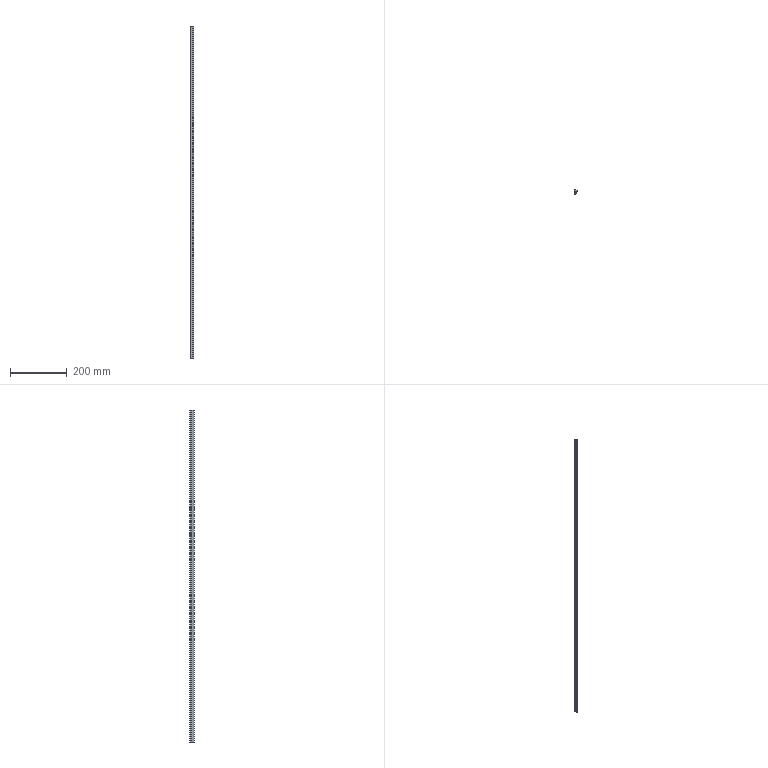Part | SolidWorks | features BaseBody 1, MoveFace 1 | 1 solid | 20 faces | box 10.8 x 17.5 x 1171 mm | volume 92275 mm3 | cylinder 11 | plane 9 | commonest cylinder face diameters 1.6 x2 14 x2 0.4 x1 0.6 x1 0.8 x1 2.6 x1
STEP:
#1=CARTESIAN_POINT('',(-3.236,-11.055,1071.));
#2=VERTEX_POINT('',#1);
#3=CARTESIAN_POINT('',(-4.3,-10.3,1071.));
#4=VERTEX_POINT('',#3);
#5=CARTESIAN_POINT('',(-3.5,-10.3,1071.));
#6=DIRECTION('',(0.,0.,-1.));
#7=DIRECTION('',(1.,0.,0.));
#8=AXIS2_PLACEMENT_3D('',#5,#6,#7);
#9=CIRCLE('',#8,0.8);
#10=EDGE_CURVE('',#2,#4,#9,.T.);
#11=ORIENTED_EDGE('',*,*,#10,.T.);
#12=CARTESIAN_POINT('',(-4.3,-10.3,-100.));
#13=VERTEX_POINT('',#12);
#14=CARTESIAN_POINT('',(-4.3,-10.3,-100.));
#15=DIRECTION('',(0.,0.,-1.));
#16=VECTOR('',#15,1000.);
#17=LINE('',#14,#16);
#18=EDGE_CURVE('',#4,#13,#17,.T.);
#19=ORIENTED_EDGE('',*,*,#18,.T.);
#20=CARTESIAN_POINT('',(-3.236,-11.055,-100.));
#21=VERTEX_POINT('',#20);
#22=CARTESIAN_POINT('',(-3.5,-10.3,-100.));
#23=DIRECTION('',(0.,0.,1.));
#24=DIRECTION('',(-1.,0.,0.));
#25=AXIS2_PLACEMENT_3D('',#22,#23,#24);
#26=CIRCLE('',#25,0.8);
#27=EDGE_CURVE('',#13,#21,#26,.T.);
#28=ORIENTED_EDGE('',*,*,#27,.T.);
#29=CARTESIAN_POINT('',(-3.236,-11.055,-100.));
#30=DIRECTION('',(0.,0.,-1.));
#31=VECTOR('',#30,1000.);
#32=LINE('',#29,#31);
#33=EDGE_CURVE('',#2,#21,#32,.T.);
#34=ORIENTED_EDGE('',*,*,#33,.F.);
#35=EDGE_LOOP('',(#11,#19,#28,#34));
#36=FACE_OUTER_BOUND('',#35,.T.);
#37=CARTESIAN_POINT('',(-3.5,-10.3,-100.));
#38=DIRECTION('',(0.,0.,-1.));
#39=DIRECTION('',(-1.,0.,0.));
#40=AXIS2_PLACEMENT_3D('',#37,#38,#39);
#41=CYLINDRICAL_SURFACE('',#40,0.8);
#42=ADVANCED_FACE('',(#36),#41,.T.);
#43=CARTESIAN_POINT('',(1.184,-6.397,-100.));
#44=VERTEX_POINT('',#43);
#45=CARTESIAN_POINT('',(-5.702,-4.29,-100.));
#46=DIRECTION('',(0.,0.,1.));
#47=DIRECTION('',(-1.,0.,0.));
#48=AXIS2_PLACEMENT_3D('',#45,#46,#47);
#49=CIRCLE('',#48,7.201);
#50=EDGE_CURVE('',#21,#44,#49,.T.);
#51=ORIENTED_EDGE('',*,*,#50,.T.);
#52=CARTESIAN_POINT('',(1.184,-6.397,1071.));
#53=VERTEX_POINT('',#52);
#54=CARTESIAN_POINT('',(1.184,-6.397,-100.));
#55=DIRECTION('',(0.,0.,1.));
#56=VECTOR('',#55,1000.);
#57=LINE('',#54,#56);
#58=EDGE_CURVE('',#44,#53,#57,.T.);
#59=ORIENTED_EDGE('',*,*,#58,.T.);
#60=CARTESIAN_POINT('',(-5.702,-4.29,1071.));
#61=DIRECTION('',(0.,0.,-1.));
#62=DIRECTION('',(1.,0.,0.));
#63=AXIS2_PLACEMENT_3D('',#60,#61,#62);
#64=CIRCLE('',#63,7.201);
#65=EDGE_CURVE('',#53,#2,#64,.T.);
#66=ORIENTED_EDGE('',*,*,#65,.T.);
#67=ORIENTED_EDGE('',*,*,#33,.T.);
#68=EDGE_LOOP('',(#51,#59,#66,#67));
#69=FACE_OUTER_BOUND('',#68,.T.);
#70=CARTESIAN_POINT('',(-5.702,-4.29,-100.));
#71=DIRECTION('',(0.,0.,-1.));
#72=DIRECTION('',(-1.,0.,0.));
#73=AXIS2_PLACEMENT_3D('',#70,#71,#72);
#74=CYLINDRICAL_SURFACE('',#73,7.201);
#75=ADVANCED_FACE('',(#69),#74,.T.);
#76=CARTESIAN_POINT('',(0.9,-6.,-100.));
#77=VERTEX_POINT('',#76);
#78=CARTESIAN_POINT('',(0.9,-6.3,-100.));
#79=DIRECTION('',(0.,0.,1.));
#80=DIRECTION('',(-1.,0.,0.));
#81=AXIS2_PLACEMENT_3D('',#78,#79,#80);
#82=CIRCLE('',#81,0.3);
#83=EDGE_CURVE('',#44,#77,#82,.T.);
#84=ORIENTED_EDGE('',*,*,#83,.T.);
#85=CARTESIAN_POINT('',(0.9,-6.,1071.));
#86=VERTEX_POINT('',#85);
#87=CARTESIAN_POINT('',(0.9,-6.,-100.));
#88=DIRECTION('',(0.,0.,1.));
#89=VECTOR('',#88,1000.);
#90=LINE('',#87,#89);
#91=EDGE_CURVE('',#77,#86,#90,.T.);
#92=ORIENTED_EDGE('',*,*,#91,.T.);
#93=CARTESIAN_POINT('',(0.9,-6.3,1071.));
#94=DIRECTION('',(0.,0.,-1.));
#95=DIRECTION('',(1.,0.,0.));
#96=AXIS2_PLACEMENT_3D('',#93,#94,#95);
#97=CIRCLE('',#96,0.3);
#98=EDGE_CURVE('',#86,#53,#97,.T.);
#99=ORIENTED_EDGE('',*,*,#98,.T.);
#100=ORIENTED_EDGE('',*,*,#58,.F.);
#101=EDGE_LOOP('',(#84,#92,#99,#100));
#102=FACE_OUTER_BOUND('',#101,.T.);
#103=CARTESIAN_POINT('',(0.9,-6.3,-100.));
#104=DIRECTION('',(0.,0.,-1.));
#105=DIRECTION('',(-1.,0.,0.));
#106=AXIS2_PLACEMENT_3D('',#103,#104,#105);
#107=CYLINDRICAL_SURFACE('',#106,0.3);
#108=ADVANCED_FACE('',(#102),#107,.T.);
#109=CARTESIAN_POINT('',(-2.5,-0.5,-100.));
#110=VERTEX_POINT('',#109);
#111=CARTESIAN_POINT('',(-2.5,-6.153,-100.));
#112=VERTEX_POINT('',#111);
#113=CARTESIAN_POINT('',(-2.5,-6.397,-100.));
#114=DIRECTION('',(0.,-1.,0.));
#115=VECTOR('',#114,1000.);
#116=LINE('',#113,#115);
#117=EDGE_CURVE('',#110,#112,#116,.T.);
#118=ORIENTED_EDGE('',*,*,#117,.F.);
#119=CARTESIAN_POINT('',(-4.2,1.695,-100.));
#120=VERTEX_POINT('',#119);
#121=CARTESIAN_POINT('',(-1.701,1.875,-100.));
#122=DIRECTION('',(0.,0.,1.));
#123=DIRECTION('',(-1.,0.,0.));
#124=AXIS2_PLACEMENT_3D('',#121,#122,#123);
#125=CIRCLE('',#124,2.506);
#126=EDGE_CURVE('',#120,#110,#125,.T.);
#127=ORIENTED_EDGE('',*,*,#126,.F.);
#128=CARTESIAN_POINT('',(-4.2,5.1,-100.));
#129=VERTEX_POINT('',#128);
#130=CARTESIAN_POINT('',(-4.2,-6.397,-100.));
#131=DIRECTION('',(0.,-1.,0.));
#132=VECTOR('',#131,1000.);
#133=LINE('',#130,#132);
#134=EDGE_CURVE('',#129,#120,#133,.T.);
#135=ORIENTED_EDGE('',*,*,#134,.F.);
#136=CARTESIAN_POINT('',(-2.892,6.4,-100.));
#137=VERTEX_POINT('',#136);
#138=CARTESIAN_POINT('',(-2.9,5.1,-100.));
#139=DIRECTION('',(0.,0.,1.));
#140=DIRECTION('',(-1.,0.,0.));
#141=AXIS2_PLACEMENT_3D('',#138,#139,#140);
#142=CIRCLE('',#141,1.3);
#143=EDGE_CURVE('',#137,#129,#142,.T.);
#144=ORIENTED_EDGE('',*,*,#143,.F.);
#145=CARTESIAN_POINT('',(0.5,5.5,-100.));
#146=VERTEX_POINT('',#145);
#147=CARTESIAN_POINT('',(-2.934,-0.5999,-100.));
#148=DIRECTION('',(0.,0.,1.));
#149=DIRECTION('',(-1.,0.,0.));
#150=AXIS2_PLACEMENT_3D('',#147,#148,#149);
#151=CIRCLE('',#150,7.);
#152=EDGE_CURVE('',#146,#137,#151,.T.);
#153=ORIENTED_EDGE('',*,*,#152,.F.);
#154=CARTESIAN_POINT('',(5.5,1.7,-100.));
#155=VERTEX_POINT('',#154);
#156=CARTESIAN_POINT('',(5.5,1.7,-100.));
#157=DIRECTION('',(-0.7962,0.6051,0.));
#158=VECTOR('',#157,1000.);
#159=LINE('',#156,#158);
#160=EDGE_CURVE('',#155,#146,#159,.T.);
#161=ORIENTED_EDGE('',*,*,#160,.F.);
#162=CARTESIAN_POINT('',(6.458,-0.2215,-100.));
#163=VERTEX_POINT('',#162);
#164=CARTESIAN_POINT('',(6.458,-0.2215,-100.));
#165=DIRECTION('',(-0.4462,0.8949,0.));
#166=VECTOR('',#165,1000.);
#167=LINE('',#164,#166);
#168=EDGE_CURVE('',#163,#155,#167,.T.);
#169=ORIENTED_EDGE('',*,*,#168,.F.);
#170=CARTESIAN_POINT('',(5.895,-0.7433,-100.));
#171=VERTEX_POINT('',#170);
#172=CARTESIAN_POINT('',(6.1,-0.4,-100.));
#173=DIRECTION('',(0.,0.,1.));
#174=DIRECTION('',(-1.,0.,0.));
#175=AXIS2_PLACEMENT_3D('',#172,#173,#174);
#176=CIRCLE('',#175,0.4);
#177=EDGE_CURVE('',#171,#163,#176,.T.);
#178=ORIENTED_EDGE('',*,*,#177,.F.);
#179=CARTESIAN_POINT('',(3.,0.,-100.));
#180=VERTEX_POINT('',#179);
#181=CARTESIAN_POINT('',(2.746,-6.995,-100.));
#182=DIRECTION('',(0.,0.,-1.));
#183=DIRECTION('',(-1.,0.,0.));
#184=AXIS2_PLACEMENT_3D('',#181,#182,#183);
#185=CIRCLE('',#184,7.);
#186=EDGE_CURVE('',#180,#171,#185,.T.);
#187=ORIENTED_EDGE('',*,*,#186,.F.);
#188=CARTESIAN_POINT('',(0.,0.,-100.));
#189=VERTEX_POINT('',#188);
#190=CARTESIAN_POINT('',(-6.814,0.,-100.));
#191=DIRECTION('',(1.,0.,0.));
#192=VECTOR('',#191,1000.);
#193=LINE('',#190,#192);
#194=EDGE_CURVE('',#189,#180,#193,.T.);
#195=ORIENTED_EDGE('',*,*,#194,.F.);
#196=CARTESIAN_POINT('',(0.,-5.8,-100.));
#197=VERTEX_POINT('',#196);
#198=CARTESIAN_POINT('',(0.,-6.397,-100.));
#199=DIRECTION('',(0.,1.,0.));
#200=VECTOR('',#199,1000.);
#201=LINE('',#198,#200);
#202=EDGE_CURVE('',#197,#189,#201,.T.);
#203=ORIENTED_EDGE('',*,*,#202,.F.);
#204=CARTESIAN_POINT('',(0.2,-6.,-100.));
#205=VERTEX_POINT('',#204);
#206=CARTESIAN_POINT('',(0.2,-5.8,-100.));
#207=DIRECTION('',(0.,0.,1.));
#208=DIRECTION('',(-1.,0.,0.));
#209=AXIS2_PLACEMENT_3D('',#206,#207,#208);
#210=CIRCLE('',#209,0.2);
#211=EDGE_CURVE('',#197,#205,#210,.T.);
#212=ORIENTED_EDGE('',*,*,#211,.T.);
#213=CARTESIAN_POINT('',(-6.814,-6.,-100.));
#214=DIRECTION('',(-1.,0.,0.));
#215=VECTOR('',#214,1000.);
#216=LINE('',#213,#215);
#217=EDGE_CURVE('',#77,#205,#216,.T.);
#218=ORIENTED_EDGE('',*,*,#217,.F.);
#219=ORIENTED_EDGE('',*,*,#83,.F.);
#220=ORIENTED_EDGE('',*,*,#50,.F.);
#221=ORIENTED_EDGE('',*,*,#27,.F.);
#222=CARTESIAN_POINT('',(-3.998,-9.674,-100.));
#223=VERTEX_POINT('',#222);
#224=CARTESIAN_POINT('',(-3.5,-10.3,-100.));
#225=DIRECTION('',(0.,0.,1.));
#226=DIRECTION('',(-1.,0.,0.));
#227=AXIS2_PLACEMENT_3D('',#224,#225,#226);
#228=CIRCLE('',#227,0.8);
#229=EDGE_CURVE('',#223,#13,#228,.T.);
#230=ORIENTED_EDGE('',*,*,#229,.F.);
#231=CARTESIAN_POINT('',(-6.814,-6.397,-100.));
#232=DIRECTION('',(0.,0.,-1.));
#233=DIRECTION('',(-1.,0.,0.));
#234=AXIS2_PLACEMENT_3D('',#231,#232,#233);
#235=CIRCLE('',#234,4.321);
#236=EDGE_CURVE('',#112,#223,#235,.T.);
#237=ORIENTED_EDGE('',*,*,#236,.F.);
#238=EDGE_LOOP('',(#118,#127,#135,#144,#153,#161,#169,#178,#187,#195,#203,#212,#218,#219,#220,#221,#230,#237));
#239=FACE_OUTER_BOUND('',#238,.T.);
#240=CARTESIAN_POINT('',(-6.814,-6.397,-100.));
#241=DIRECTION('',(0.,0.,1.));
#242=DIRECTION('',(1.,0.,0.));
#243=AXIS2_PLACEMENT_3D('',#240,#241,#242);
#244=PLANE('',#243);
#245=ADVANCED_FACE('',(#239),#244,.F.);
#246=ORIENTED_EDGE('',*,*,#18,.F.);
#247=CARTESIAN_POINT('',(-3.998,-9.674,1071.));
#248=VERTEX_POINT('',#247);
#249=CARTESIAN_POINT('',(-3.5,-10.3,1071.));
#250=DIRECTION('',(0.,0.,-1.));
#251=DIRECTION('',(1.,0.,0.));
#252=AXIS2_PLACEMENT_3D('',#249,#250,#251);
#253=CIRCLE('',#252,0.8);
#254=EDGE_CURVE('',#4,#248,#253,.T.);
#255=ORIENTED_EDGE('',*,*,#254,.T.);
#256=CARTESIAN_POINT('',(-3.998,-9.674,-100.));
#257=DIRECTION('',(0.,0.,-1.));
#258=VECTOR('',#257,1000.);
#259=LINE('',#256,#258);
#260=EDGE_CURVE('',#248,#223,#259,.T.);
#261=ORIENTED_EDGE('',*,*,#260,.T.);
#262=ORIENTED_EDGE('',*,*,#229,.T.);
#263=EDGE_LOOP('',(#246,#255,#261,#262));
#264=FACE_OUTER_BOUND('',#263,.T.);
#265=CARTESIAN_POINT('',(-3.5,-10.3,-100.));
#266=DIRECTION('',(0.,0.,-1.));
#267=DIRECTION('',(-1.,0.,0.));
#268=AXIS2_PLACEMENT_3D('',#265,#266,#267);
#269=CYLINDRICAL_SURFACE('',#268,0.8);
#270=ADVANCED_FACE('',(#264),#269,.T.);
#271=CARTESIAN_POINT('',(-4.2,1.695,1071.));
#272=VERTEX_POINT('',#271);
#273=CARTESIAN_POINT('',(-2.5,-0.5,1071.));
#274=VERTEX_POINT('',#273);
#275=CARTESIAN_POINT('',(-1.701,1.875,1071.));
#276=DIRECTION('',(0.,0.,1.));
#277=DIRECTION('',(1.,0.,0.));
#278=AXIS2_PLACEMENT_3D('',#275,#276,#277);
#279=CIRCLE('',#278,2.506);
#280=EDGE_CURVE('',#272,#274,#279,.T.);
#281=ORIENTED_EDGE('',*,*,#280,.T.);
#282=CARTESIAN_POINT('',(-2.5,-6.153,1071.));
#283=VERTEX_POINT('',#282);
#284=CARTESIAN_POINT('',(-2.5,-6.397,1071.));
#285=DIRECTION('',(0.,-1.,0.));
#286=VECTOR('',#285,1000.);
#287=LINE('',#284,#286);
#288=EDGE_CURVE('',#274,#283,#287,.T.);
#289=ORIENTED_EDGE('',*,*,#288,.T.);
#290=CARTESIAN_POINT('',(-6.814,-6.397,1071.));
#291=DIRECTION('',(0.,0.,-1.));
#292=DIRECTION('',(1.,0.,0.));
#293=AXIS2_PLACEMENT_3D('',#290,#291,#292);
#294=CIRCLE('',#293,4.321);
#295=EDGE_CURVE('',#283,#248,#294,.T.);
#296=ORIENTED_EDGE('',*,*,#295,.T.);
#297=ORIENTED_EDGE('',*,*,#254,.F.);
#298=ORIENTED_EDGE('',*,*,#10,.F.);
#299=ORIENTED_EDGE('',*,*,#65,.F.);
#300=ORIENTED_EDGE('',*,*,#98,.F.);
#301=CARTESIAN_POINT('',(0.2,-6.,1071.));
#302=VERTEX_POINT('',#301);
#303=CARTESIAN_POINT('',(-6.814,-6.,1071.));
#304=DIRECTION('',(-1.,0.,0.));
#305=VECTOR('',#304,1000.);
#306=LINE('',#303,#305);
#307=EDGE_CURVE('',#86,#302,#306,.T.);
#308=ORIENTED_EDGE('',*,*,#307,.T.);
#309=CARTESIAN_POINT('',(0.,-5.8,1071.));
#310=VERTEX_POINT('',#309);
#311=CARTESIAN_POINT('',(0.2,-5.8,1071.));
#312=DIRECTION('',(0.,0.,-1.));
#313=DIRECTION('',(1.,0.,0.));
#314=AXIS2_PLACEMENT_3D('',#311,#312,#313);
#315=CIRCLE('',#314,0.2);
#316=EDGE_CURVE('',#302,#310,#315,.T.);
#317=ORIENTED_EDGE('',*,*,#316,.T.);
#318=CARTESIAN_POINT('',(0.,0.,1071.));
#319=VERTEX_POINT('',#318);
#320=CARTESIAN_POINT('',(0.,-6.397,1071.));
#321=DIRECTION('',(0.,1.,0.));
#322=VECTOR('',#321,1000.);
#323=LINE('',#320,#322);
#324=EDGE_CURVE('',#310,#319,#323,.T.);
#325=ORIENTED_EDGE('',*,*,#324,.T.);
#326=CARTESIAN_POINT('',(3.,0.,1071.));
#327=VERTEX_POINT('',#326);
#328=CARTESIAN_POINT('',(-6.814,0.,1071.));
#329=DIRECTION('',(1.,0.,0.));
#330=VECTOR('',#329,1000.);
#331=LINE('',#328,#330);
#332=EDGE_CURVE('',#319,#327,#331,.T.);
#333=ORIENTED_EDGE('',*,*,#332,.T.);
#334=CARTESIAN_POINT('',(5.895,-0.7433,1071.));
#335=VERTEX_POINT('',#334);
#336=CARTESIAN_POINT('',(2.746,-6.995,1071.));
#337=DIRECTION('',(0.,0.,-1.));
#338=DIRECTION('',(1.,0.,0.));
#339=AXIS2_PLACEMENT_3D('',#336,#337,#338);
#340=CIRCLE('',#339,7.);
#341=EDGE_CURVE('',#327,#335,#340,.T.);
#342=ORIENTED_EDGE('',*,*,#341,.T.);
#343=CARTESIAN_POINT('',(6.458,-0.2215,1071.));
#344=VERTEX_POINT('',#343);
#345=CARTESIAN_POINT('',(6.1,-0.4,1071.));
#346=DIRECTION('',(0.,0.,-1.));
#347=DIRECTION('',(1.,0.,0.));
#348=AXIS2_PLACEMENT_3D('',#345,#346,#347);
#349=CIRCLE('',#348,0.4);
#350=EDGE_CURVE('',#344,#335,#349,.T.);
#351=ORIENTED_EDGE('',*,*,#350,.F.);
#352=CARTESIAN_POINT('',(5.5,1.7,1071.));
#353=VERTEX_POINT('',#352);
#354=CARTESIAN_POINT('',(6.282,0.1323,1071.));
#355=DIRECTION('',(-0.4462,0.8949,0.));
#356=VECTOR('',#355,1000.);
#357=LINE('',#354,#356);
#358=EDGE_CURVE('',#344,#353,#357,.T.);
#359=ORIENTED_EDGE('',*,*,#358,.T.);
#360=CARTESIAN_POINT('',(0.5,5.5,1071.));
#361=VERTEX_POINT('',#360);
#362=CARTESIAN_POINT('',(1.595,4.668,1071.));
#363=DIRECTION('',(-0.7962,0.6051,0.));
#364=VECTOR('',#363,1000.);
#365=LINE('',#362,#364);
#366=EDGE_CURVE('',#353,#361,#365,.T.);
#367=ORIENTED_EDGE('',*,*,#366,.T.);
#368=CARTESIAN_POINT('',(-2.892,6.4,1071.));
#369=VERTEX_POINT('',#368);
#370=CARTESIAN_POINT('',(-2.934,-0.5999,1071.));
#371=DIRECTION('',(0.,0.,1.));
#372=DIRECTION('',(1.,0.,0.));
#373=AXIS2_PLACEMENT_3D('',#370,#371,#372);
#374=CIRCLE('',#373,7.);
#375=EDGE_CURVE('',#361,#369,#374,.T.);
#376=ORIENTED_EDGE('',*,*,#375,.T.);
#377=CARTESIAN_POINT('',(-4.2,5.1,1071.));
#378=VERTEX_POINT('',#377);
#379=CARTESIAN_POINT('',(-2.9,5.1,1071.));
#380=DIRECTION('',(0.,0.,1.));
#381=DIRECTION('',(1.,0.,0.));
#382=AXIS2_PLACEMENT_3D('',#379,#380,#381);
#383=CIRCLE('',#382,1.3);
#384=EDGE_CURVE('',#369,#378,#383,.T.);
#385=ORIENTED_EDGE('',*,*,#384,.T.);
#386=CARTESIAN_POINT('',(-4.2,-6.397,1071.));
#387=DIRECTION('',(0.,-1.,0.));
#388=VECTOR('',#387,1000.);
#389=LINE('',#386,#388);
#390=EDGE_CURVE('',#378,#272,#389,.T.);
#391=ORIENTED_EDGE('',*,*,#390,.T.);
#392=EDGE_LOOP('',(#281,#289,#296,#297,#298,#299,#300,#308,#317,#325,#333,#342,#351,#359,#367,#376,#385,#391));
#393=FACE_OUTER_BOUND('',#392,.T.);
#394=CARTESIAN_POINT('',(-6.814,-6.397,1071.));
#395=DIRECTION('',(0.,0.,1.));
#396=DIRECTION('',(1.,0.,0.));
#397=AXIS2_PLACEMENT_3D('',#394,#395,#396);
#398=PLANE('',#397);
#399=ADVANCED_FACE('',(#393),#398,.T.);
#400=ORIENTED_EDGE('',*,*,#217,.T.);
#401=CARTESIAN_POINT('',(0.2,-6.,-100.));
#402=DIRECTION('',(0.,0.,1.));
#403=VECTOR('',#402,1000.);
#404=LINE('',#401,#403);
#405=EDGE_CURVE('',#205,#302,#404,.T.);
#406=ORIENTED_EDGE('',*,*,#405,.T.);
#407=ORIENTED_EDGE('',*,*,#307,.F.);
#408=ORIENTED_EDGE('',*,*,#91,.F.);
#409=EDGE_LOOP('',(#400,#406,#407,#408));
#410=FACE_OUTER_BOUND('',#409,.T.);
#411=CARTESIAN_POINT('',(0.9,-6.,-100.));
#412=DIRECTION('',(0.,1.,0.));
#413=DIRECTION('',(0.,0.,1.));
#414=AXIS2_PLACEMENT_3D('',#411,#412,#413);
#415=PLANE('',#414);
#416=ADVANCED_FACE('',(#410),#415,.T.);
#417=CARTESIAN_POINT('',(-2.5,-6.153,-100.));
#418=DIRECTION('',(0.,0.,1.));
#419=VECTOR('',#418,1000.);
#420=LINE('',#417,#419);
#421=EDGE_CURVE('',#112,#283,#420,.T.);
#422=ORIENTED_EDGE('',*,*,#421,.F.);
#423=ORIENTED_EDGE('',*,*,#236,.T.);
#424=ORIENTED_EDGE('',*,*,#260,.F.);
#425=ORIENTED_EDGE('',*,*,#295,.F.);
#426=EDGE_LOOP('',(#422,#423,#424,#425));
#427=FACE_OUTER_BOUND('',#426,.T.);
#428=CARTESIAN_POINT('',(-6.814,-6.397,-100.));
#429=DIRECTION('',(0.,0.,-1.));
#430=DIRECTION('',(-1.,0.,0.));
#431=AXIS2_PLACEMENT_3D('',#428,#429,#430);
#432=CYLINDRICAL_SURFACE('',#431,4.321);
#433=ADVANCED_FACE('',(#427),#432,.F.);
#434=ORIENTED_EDGE('',*,*,#117,.T.);
#435=ORIENTED_EDGE('',*,*,#421,.T.);
#436=ORIENTED_EDGE('',*,*,#288,.F.);
#437=CARTESIAN_POINT('',(-2.5,-0.5,-100.));
#438=DIRECTION('',(0.,0.,-1.));
#439=VECTOR('',#438,1000.);
#440=LINE('',#437,#439);
#441=EDGE_CURVE('',#274,#110,#440,.T.);
#442=ORIENTED_EDGE('',*,*,#441,.T.);
#443=EDGE_LOOP('',(#434,#435,#436,#442));
#444=FACE_OUTER_BOUND('',#443,.T.);
#445=CARTESIAN_POINT('',(-2.5,-0.5,-100.));
#446=DIRECTION('',(-1.,0.,0.));
#447=DIRECTION('',(0.,0.,1.));
#448=AXIS2_PLACEMENT_3D('',#445,#446,#447);
#449=PLANE('',#448);
#450=ADVANCED_FACE('',(#444),#449,.T.);
#451=ORIENTED_EDGE('',*,*,#126,.T.);
#452=ORIENTED_EDGE('',*,*,#441,.F.);
#453=ORIENTED_EDGE('',*,*,#280,.F.);
#454=CARTESIAN_POINT('',(-4.2,1.695,-100.));
#455=DIRECTION('',(0.,0.,-1.));
#456=VECTOR('',#455,1000.);
#457=LINE('',#454,#456);
#458=EDGE_CURVE('',#272,#120,#457,.T.);
#459=ORIENTED_EDGE('',*,*,#458,.T.);
#460=EDGE_LOOP('',(#451,#452,#453,#459));
#461=FACE_OUTER_BOUND('',#460,.T.);
#462=CARTESIAN_POINT('',(-1.701,1.875,-100.));
#463=DIRECTION('',(0.,0.,-1.));
#464=DIRECTION('',(-1.,0.,0.));
#465=AXIS2_PLACEMENT_3D('',#462,#463,#464);
#466=CYLINDRICAL_SURFACE('',#465,2.506);
#467=ADVANCED_FACE('',(#461),#466,.T.);
#468=ORIENTED_EDGE('',*,*,#134,.T.);
#469=ORIENTED_EDGE('',*,*,#458,.F.);
#470=ORIENTED_EDGE('',*,*,#390,.F.);
#471=CARTESIAN_POINT('',(-4.2,5.1,-100.));
#472=DIRECTION('',(0.,0.,-1.));
#473=VECTOR('',#472,1000.);
#474=LINE('',#471,#473);
#475=EDGE_CURVE('',#378,#129,#474,.T.);
#476=ORIENTED_EDGE('',*,*,#475,.T.);
#477=EDGE_LOOP('',(#468,#469,#470,#476));
#478=FACE_OUTER_BOUND('',#477,.T.);
#479=CARTESIAN_POINT('',(-4.2,5.1,-100.));
#480=DIRECTION('',(-1.,0.,0.));
#481=DIRECTION('',(0.,0.,1.));
#482=AXIS2_PLACEMENT_3D('',#479,#480,#481);
#483=PLANE('',#482);
#484=ADVANCED_FACE('',(#478),#483,.T.);
#485=ORIENTED_EDGE('',*,*,#143,.T.);
#486=ORIENTED_EDGE('',*,*,#475,.F.);
#487=ORIENTED_EDGE('',*,*,#384,.F.);
#488=CARTESIAN_POINT('',(-2.892,6.4,-100.));
#489=DIRECTION('',(0.,0.,-1.));
#490=VECTOR('',#489,1000.);
#491=LINE('',#488,#490);
#492=EDGE_CURVE('',#369,#137,#491,.T.);
#493=ORIENTED_EDGE('',*,*,#492,.T.);
#494=EDGE_LOOP('',(#485,#486,#487,#493));
#495=FACE_OUTER_BOUND('',#494,.T.);
#496=CARTESIAN_POINT('',(-2.9,5.1,-100.));
#497=DIRECTION('',(0.,0.,-1.));
#498=DIRECTION('',(-1.,0.,0.));
#499=AXIS2_PLACEMENT_3D('',#496,#497,#498);
#500=CYLINDRICAL_SURFACE('',#499,1.3);
#501=ADVANCED_FACE('',(#495),#500,.T.);
#502=ORIENTED_EDGE('',*,*,#152,.T.);
#503=ORIENTED_EDGE('',*,*,#492,.F.);
#504=ORIENTED_EDGE('',*,*,#375,.F.);
#505=CARTESIAN_POINT('',(0.5,5.5,-100.));
#506=DIRECTION('',(0.,0.,-1.));
#507=VECTOR('',#506,1000.);
#508=LINE('',#505,#507);
#509=EDGE_CURVE('',#361,#146,#508,.T.);
#510=ORIENTED_EDGE('',*,*,#509,.T.);
#511=EDGE_LOOP('',(#502,#503,#504,#510));
#512=FACE_OUTER_BOUND('',#511,.T.);
#513=CARTESIAN_POINT('',(-2.934,-0.5999,-100.));
#514=DIRECTION('',(0.,0.,-1.));
#515=DIRECTION('',(-1.,0.,0.));
#516=AXIS2_PLACEMENT_3D('',#513,#514,#515);
#517=CYLINDRICAL_SURFACE('',#516,7.);
#518=ADVANCED_FACE('',(#512),#517,.T.);
#519=ORIENTED_EDGE('',*,*,#160,.T.);
#520=ORIENTED_EDGE('',*,*,#509,.F.);
#521=ORIENTED_EDGE('',*,*,#366,.F.);
#522=CARTESIAN_POINT('',(5.5,1.7,-100.));
#523=DIRECTION('',(0.,0.,-1.));
#524=VECTOR('',#523,1000.);
#525=LINE('',#522,#524);
#526=EDGE_CURVE('',#353,#155,#525,.T.);
#527=ORIENTED_EDGE('',*,*,#526,.T.);
#528=EDGE_LOOP('',(#519,#520,#521,#527));
#529=FACE_OUTER_BOUND('',#528,.T.);
#530=CARTESIAN_POINT('',(5.5,1.7,-100.));
#531=DIRECTION('',(0.6051,0.7962,0.));
#532=DIRECTION('',(-0.7962,0.6051,0.));
#533=AXIS2_PLACEMENT_3D('',#530,#531,#532);
#534=PLANE('',#533);
#535=ADVANCED_FACE('',(#529),#534,.T.);
#536=ORIENTED_EDGE('',*,*,#168,.T.);
#537=ORIENTED_EDGE('',*,*,#526,.F.);
#538=ORIENTED_EDGE('',*,*,#358,.F.);
#539=CARTESIAN_POINT('',(6.458,-0.2215,-100.));
#540=DIRECTION('',(0.,0.,-1.));
#541=VECTOR('',#540,1000.);
#542=LINE('',#539,#541);
#543=EDGE_CURVE('',#344,#163,#542,.T.);
#544=ORIENTED_EDGE('',*,*,#543,.T.);
#545=EDGE_LOOP('',(#536,#537,#538,#544));
#546=FACE_OUTER_BOUND('',#545,.T.);
#547=CARTESIAN_POINT('',(6.458,-0.2215,-100.));
#548=DIRECTION('',(0.8949,0.4462,0.));
#549=DIRECTION('',(-0.4462,0.8949,0.));
#550=AXIS2_PLACEMENT_3D('',#547,#548,#549);
#551=PLANE('',#550);
#552=ADVANCED_FACE('',(#546),#551,.T.);
#553=CARTESIAN_POINT('',(3.,0.,-100.));
#554=DIRECTION('',(0.,0.,1.));
#555=VECTOR('',#554,1000.);
#556=LINE('',#553,#555);
#557=EDGE_CURVE('',#180,#327,#556,.T.);
#558=ORIENTED_EDGE('',*,*,#557,.F.);
#559=ORIENTED_EDGE('',*,*,#186,.T.);
#560=CARTESIAN_POINT('',(5.895,-0.7433,-100.));
#561=DIRECTION('',(0.,0.,-1.));
#562=VECTOR('',#561,1000.);
#563=LINE('',#560,#562);
#564=EDGE_CURVE('',#335,#171,#563,.T.);
#565=ORIENTED_EDGE('',*,*,#564,.F.);
#566=ORIENTED_EDGE('',*,*,#341,.F.);
#567=EDGE_LOOP('',(#558,#559,#565,#566));
#568=FACE_OUTER_BOUND('',#567,.T.);
#569=CARTESIAN_POINT('',(2.746,-6.995,-100.));
#570=DIRECTION('',(0.,0.,-1.));
#571=DIRECTION('',(-1.,0.,0.));
#572=AXIS2_PLACEMENT_3D('',#569,#570,#571);
#573=CYLINDRICAL_SURFACE('',#572,7.);
#574=ADVANCED_FACE('',(#568),#573,.F.);
#575=ORIENTED_EDGE('',*,*,#194,.T.);
#576=ORIENTED_EDGE('',*,*,#557,.T.);
#577=ORIENTED_EDGE('',*,*,#332,.F.);
#578=CARTESIAN_POINT('',(0.,0.,-100.));
#579=DIRECTION('',(0.,0.,-1.));
#580=VECTOR('',#579,1000.);
#581=LINE('',#578,#580);
#582=EDGE_CURVE('',#319,#189,#581,.T.);
#583=ORIENTED_EDGE('',*,*,#582,.T.);
#584=EDGE_LOOP('',(#575,#576,#577,#583));
#585=FACE_OUTER_BOUND('',#584,.T.);
#586=CARTESIAN_POINT('',(0.,0.,-100.));
#587=DIRECTION('',(0.,-1.,0.));
#588=DIRECTION('',(0.,0.,-1.));
#589=AXIS2_PLACEMENT_3D('',#586,#587,#588);
#590=PLANE('',#589);
#591=ADVANCED_FACE('',(#585),#590,.T.);
#592=ORIENTED_EDGE('',*,*,#202,.T.);
#593=ORIENTED_EDGE('',*,*,#582,.F.);
#594=ORIENTED_EDGE('',*,*,#324,.F.);
#595=CARTESIAN_POINT('',(0.,-5.8,-100.));
#596=DIRECTION('',(0.,0.,-1.));
#597=VECTOR('',#596,1000.);
#598=LINE('',#595,#597);
#599=EDGE_CURVE('',#310,#197,#598,.T.);
#600=ORIENTED_EDGE('',*,*,#599,.T.);
#601=EDGE_LOOP('',(#592,#593,#594,#600));
#602=FACE_OUTER_BOUND('',#601,.T.);
#603=CARTESIAN_POINT('',(0.,-5.8,-100.));
#604=DIRECTION('',(1.,0.,0.));
#605=DIRECTION('',(0.,0.,-1.));
#606=AXIS2_PLACEMENT_3D('',#603,#604,#605);
#607=PLANE('',#606);
#608=ADVANCED_FACE('',(#602),#607,.T.);
#609=ORIENTED_EDGE('',*,*,#405,.F.);
#610=ORIENTED_EDGE('',*,*,#211,.F.);
#611=ORIENTED_EDGE('',*,*,#599,.F.);
#612=ORIENTED_EDGE('',*,*,#316,.F.);
#613=EDGE_LOOP('',(#609,#610,#611,#612));
#614=FACE_OUTER_BOUND('',#613,.T.);
#615=CARTESIAN_POINT('',(0.2,-5.8,-100.));
#616=DIRECTION('',(0.,0.,-1.));
#617=DIRECTION('',(-1.,0.,0.));
#618=AXIS2_PLACEMENT_3D('',#615,#616,#617);
#619=CYLINDRICAL_SURFACE('',#618,0.2);
#620=ADVANCED_FACE('',(#614),#619,.F.);
#621=ORIENTED_EDGE('',*,*,#177,.T.);
#622=ORIENTED_EDGE('',*,*,#543,.F.);
#623=ORIENTED_EDGE('',*,*,#350,.T.);
#624=ORIENTED_EDGE('',*,*,#564,.T.);
#625=EDGE_LOOP('',(#621,#622,#623,#624));
#626=FACE_OUTER_BOUND('',#625,.T.);
#627=CARTESIAN_POINT('',(6.1,-0.4,-100.));
#628=DIRECTION('',(0.,0.,-1.));
#629=DIRECTION('',(-1.,0.,0.));
#630=AXIS2_PLACEMENT_3D('',#627,#628,#629);
#631=CYLINDRICAL_SURFACE('',#630,0.4);
#632=ADVANCED_FACE('',(#626),#631,.T.);
#633=CLOSED_SHELL('',(#42,#75,#108,#245,#270,#399,#416,#433,#450,#467,#484,#501,#518,#535,#552,#574,#591,#608,#620,#632));
#634=MANIFOLD_SOLID_BREP('',#633);
#635=CARTESIAN_POINT('',(0.,0.,0.));
#636=DIRECTION('',(0.,0.,1.));
#637=DIRECTION('',(1.,0.,0.));
#638=AXIS2_PLACEMENT_3D('',#635,#636,#637);
#639=(LENGTH_UNIT()NAMED_UNIT(*)SI_UNIT(.MILLI.,.METRE.));
#640=UNCERTAINTY_MEASURE_WITH_UNIT(LENGTH_MEASURE(0.00001),#639,'','');
#641=(NAMED_UNIT(*)PLANE_ANGLE_UNIT()SI_UNIT($,.RADIAN.));
#642=(NAMED_UNIT(*)SI_UNIT($,.STERADIAN.)SOLID_ANGLE_UNIT());
#643=(GEOMETRIC_REPRESENTATION_CONTEXT(3)GLOBAL_UNCERTAINTY_ASSIGNED_CONTEXT((#640))GLOBAL_UNIT_ASSIGNED_CONTEXT((#639,#641,#642))REPRESENTATION_CONTEXT('',''));
#644=ADVANCED_BREP_SHAPE_REPRESENTATION('',(#634,#638),#643);